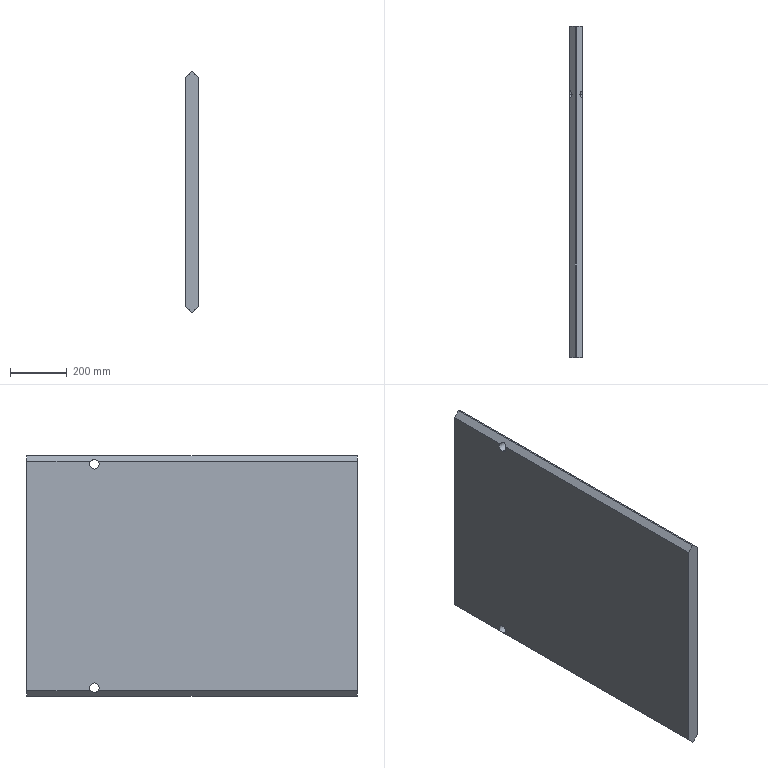Part | SolidWorks | features Chamfer 1, Extrusion 1 | 1 solid | 14 faces | box 45 x 1170 x 850 mm | volume 43736327 mm3 | plane 10 | cylinder 4 | commonest cylinder face diameters 34 x4
STEP:
#1=CARTESIAN_POINT('',(22.5,331.252,405.));
#2=VERTEX_POINT('',#1);
#3=CARTESIAN_POINT('',(22.5,345.,378.));
#4=VERTEX_POINT('',#3);
#5=CARTESIAN_POINT('',(22.5,345.,395.));
#6=DIRECTION('',(1.,0.,0.));
#7=DIRECTION('',(0.,0.,-1.));
#8=AXIS2_PLACEMENT_3D('',#5,#6,#7);
#9=CIRCLE('',#8,17.);
#10=EDGE_CURVE('',#2,#4,#9,.T.);
#11=ORIENTED_EDGE('',*,*,#10,.T.);
#12=CARTESIAN_POINT('',(-22.5,345.,378.));
#13=VERTEX_POINT('',#12);
#14=CARTESIAN_POINT('',(22.5,345.,378.));
#15=DIRECTION('',(-1.,0.,0.));
#16=VECTOR('',#15,1000.);
#17=LINE('',#14,#16);
#18=EDGE_CURVE('',#4,#13,#17,.T.);
#19=ORIENTED_EDGE('',*,*,#18,.T.);
#20=CARTESIAN_POINT('',(-22.5,331.252,405.));
#21=VERTEX_POINT('',#20);
#22=CARTESIAN_POINT('',(-22.5,345.,395.));
#23=DIRECTION('',(1.,0.,0.));
#24=DIRECTION('',(0.,0.,-1.));
#25=AXIS2_PLACEMENT_3D('',#22,#23,#24);
#26=CIRCLE('',#25,17.);
#27=EDGE_CURVE('',#21,#13,#26,.T.);
#28=ORIENTED_EDGE('',*,*,#27,.F.);
#29=CARTESIAN_POINT('',(-15.5,345.,412.));
#30=VERTEX_POINT('',#29);
#31=CARTESIAN_POINT('',(-22.5,331.252,405.));
#32=CARTESIAN_POINT('',(-18.016,334.514,409.484));
#33=CARTESIAN_POINT('',(-15.5,339.455,412.));
#34=CARTESIAN_POINT('',(-15.5,345.,412.));
#35=(BOUNDED_CURVE()B_SPLINE_CURVE(3,(#31,#32,#33,#34),.UNSPECIFIED.,.F.,.F.)B_SPLINE_CURVE_WITH_KNOTS((4,4),(2.2,3.142),.UNSPECIFIED.)CURVE()GEOMETRIC_REPRESENTATION_ITEM()RATIONAL_B_SPLINE_CURVE((1.,0.9274,0.9274,1.))REPRESENTATION_ITEM(''));
#36=EDGE_CURVE('',#21,#30,#35,.T.);
#37=ORIENTED_EDGE('',*,*,#36,.T.);
#38=CARTESIAN_POINT('',(15.5,345.,412.));
#39=VERTEX_POINT('',#38);
#40=CARTESIAN_POINT('',(22.5,345.,412.));
#41=DIRECTION('',(-1.,0.,0.));
#42=VECTOR('',#41,1000.);
#43=LINE('',#40,#42);
#44=EDGE_CURVE('',#39,#30,#43,.T.);
#45=ORIENTED_EDGE('',*,*,#44,.F.);
#46=CARTESIAN_POINT('',(15.5,345.,412.));
#47=CARTESIAN_POINT('',(15.5,339.455,412.));
#48=CARTESIAN_POINT('',(18.016,334.514,409.484));
#49=CARTESIAN_POINT('',(22.5,331.252,405.));
#50=(BOUNDED_CURVE()B_SPLINE_CURVE(3,(#46,#47,#48,#49),.UNSPECIFIED.,.F.,.T.)B_SPLINE_CURVE_WITH_KNOTS((4,4),(0.,0.9419),.UNSPECIFIED.)CURVE()GEOMETRIC_REPRESENTATION_ITEM()RATIONAL_B_SPLINE_CURVE((1.,0.9274,0.9274,1.))REPRESENTATION_ITEM(''));
#51=EDGE_CURVE('',#39,#2,#50,.T.);
#52=ORIENTED_EDGE('',*,*,#51,.T.);
#53=EDGE_LOOP('',(#11,#19,#28,#37,#45,#52));
#54=FACE_OUTER_BOUND('',#53,.T.);
#55=CARTESIAN_POINT('',(22.5,345.,395.));
#56=DIRECTION('',(-1.,0.,0.));
#57=DIRECTION('',(0.,0.,1.));
#58=AXIS2_PLACEMENT_3D('',#55,#56,#57);
#59=CYLINDRICAL_SURFACE('',#58,17.);
#60=ADVANCED_FACE('',(#54),#59,.F.);
#61=CARTESIAN_POINT('',(22.5,331.252,-405.));
#62=VERTEX_POINT('',#61);
#63=CARTESIAN_POINT('',(15.5,345.,-412.));
#64=VERTEX_POINT('',#63);
#65=CARTESIAN_POINT('',(22.5,331.252,-405.));
#66=CARTESIAN_POINT('',(18.016,334.514,-409.484));
#67=CARTESIAN_POINT('',(15.5,339.455,-412.));
#68=CARTESIAN_POINT('',(15.5,345.,-412.));
#69=(BOUNDED_CURVE()B_SPLINE_CURVE(3,(#65,#66,#67,#68),.UNSPECIFIED.,.F.,.F.)B_SPLINE_CURVE_WITH_KNOTS((4,4),(5.341,6.283),.UNSPECIFIED.)CURVE()GEOMETRIC_REPRESENTATION_ITEM()RATIONAL_B_SPLINE_CURVE((1.,0.9274,0.9274,1.))REPRESENTATION_ITEM(''));
#70=EDGE_CURVE('',#62,#64,#69,.T.);
#71=ORIENTED_EDGE('',*,*,#70,.T.);
#72=CARTESIAN_POINT('',(-15.5,345.,-412.));
#73=VERTEX_POINT('',#72);
#74=CARTESIAN_POINT('',(22.5,345.,-412.));
#75=DIRECTION('',(-1.,0.,0.));
#76=VECTOR('',#75,1000.);
#77=LINE('',#74,#76);
#78=EDGE_CURVE('',#64,#73,#77,.T.);
#79=ORIENTED_EDGE('',*,*,#78,.T.);
#80=CARTESIAN_POINT('',(-22.5,331.252,-405.));
#81=VERTEX_POINT('',#80);
#82=CARTESIAN_POINT('',(-15.5,345.,-412.));
#83=CARTESIAN_POINT('',(-15.5,339.455,-412.));
#84=CARTESIAN_POINT('',(-18.016,334.514,-409.484));
#85=CARTESIAN_POINT('',(-22.5,331.252,-405.));
#86=(BOUNDED_CURVE()B_SPLINE_CURVE(3,(#82,#83,#84,#85),.UNSPECIFIED.,.F.,.T.)B_SPLINE_CURVE_WITH_KNOTS((4,4),(3.142,4.084),.UNSPECIFIED.)CURVE()GEOMETRIC_REPRESENTATION_ITEM()RATIONAL_B_SPLINE_CURVE((1.,0.9274,0.9274,1.))REPRESENTATION_ITEM(''));
#87=EDGE_CURVE('',#73,#81,#86,.T.);
#88=ORIENTED_EDGE('',*,*,#87,.T.);
#89=CARTESIAN_POINT('',(-22.5,345.,-378.));
#90=VERTEX_POINT('',#89);
#91=CARTESIAN_POINT('',(-22.5,345.,-395.));
#92=DIRECTION('',(1.,0.,0.));
#93=DIRECTION('',(0.,0.,-1.));
#94=AXIS2_PLACEMENT_3D('',#91,#92,#93);
#95=CIRCLE('',#94,17.);
#96=EDGE_CURVE('',#90,#81,#95,.T.);
#97=ORIENTED_EDGE('',*,*,#96,.F.);
#98=CARTESIAN_POINT('',(22.5,345.,-378.));
#99=VERTEX_POINT('',#98);
#100=CARTESIAN_POINT('',(22.5,345.,-378.));
#101=DIRECTION('',(-1.,0.,0.));
#102=VECTOR('',#101,1000.);
#103=LINE('',#100,#102);
#104=EDGE_CURVE('',#99,#90,#103,.T.);
#105=ORIENTED_EDGE('',*,*,#104,.F.);
#106=CARTESIAN_POINT('',(22.5,345.,-395.));
#107=DIRECTION('',(1.,0.,0.));
#108=DIRECTION('',(0.,0.,-1.));
#109=AXIS2_PLACEMENT_3D('',#106,#107,#108);
#110=CIRCLE('',#109,17.);
#111=EDGE_CURVE('',#99,#62,#110,.T.);
#112=ORIENTED_EDGE('',*,*,#111,.T.);
#113=EDGE_LOOP('',(#71,#79,#88,#97,#105,#112));
#114=FACE_OUTER_BOUND('',#113,.T.);
#115=CARTESIAN_POINT('',(22.5,345.,-395.));
#116=DIRECTION('',(-1.,0.,0.));
#117=DIRECTION('',(0.,0.,1.));
#118=AXIS2_PLACEMENT_3D('',#115,#116,#117);
#119=CYLINDRICAL_SURFACE('',#118,17.);
#120=ADVANCED_FACE('',(#114),#119,.F.);
#121=CARTESIAN_POINT('',(22.5,-585.,405.));
#122=VERTEX_POINT('',#121);
#123=CARTESIAN_POINT('',(22.5,-585.,-405.));
#124=VERTEX_POINT('',#123);
#125=CARTESIAN_POINT('',(22.5,-585.,-425.));
#126=DIRECTION('',(0.,0.,-1.));
#127=VECTOR('',#126,1000.);
#128=LINE('',#125,#127);
#129=EDGE_CURVE('',#122,#124,#128,.T.);
#130=ORIENTED_EDGE('',*,*,#129,.T.);
#131=CARTESIAN_POINT('',(22.5,585.,-405.));
#132=DIRECTION('',(0.,1.,0.));
#133=VECTOR('',#132,1000.);
#134=LINE('',#131,#133);
#135=EDGE_CURVE('',#124,#62,#134,.T.);
#136=ORIENTED_EDGE('',*,*,#135,.T.);
#137=ORIENTED_EDGE('',*,*,#111,.F.);
#138=CARTESIAN_POINT('',(22.5,358.748,-405.));
#139=VERTEX_POINT('',#138);
#140=CARTESIAN_POINT('',(22.5,345.,-395.));
#141=DIRECTION('',(1.,0.,0.));
#142=DIRECTION('',(0.,0.,-1.));
#143=AXIS2_PLACEMENT_3D('',#140,#141,#142);
#144=CIRCLE('',#143,17.);
#145=EDGE_CURVE('',#139,#99,#144,.T.);
#146=ORIENTED_EDGE('',*,*,#145,.F.);
#147=CARTESIAN_POINT('',(22.5,585.,-405.));
#148=VERTEX_POINT('',#147);
#149=CARTESIAN_POINT('',(22.5,585.,-405.));
#150=DIRECTION('',(0.,1.,0.));
#151=VECTOR('',#150,1000.);
#152=LINE('',#149,#151);
#153=EDGE_CURVE('',#139,#148,#152,.T.);
#154=ORIENTED_EDGE('',*,*,#153,.T.);
#155=CARTESIAN_POINT('',(22.5,585.,405.));
#156=VERTEX_POINT('',#155);
#157=CARTESIAN_POINT('',(22.5,585.,-425.));
#158=DIRECTION('',(0.,0.,1.));
#159=VECTOR('',#158,1000.);
#160=LINE('',#157,#159);
#161=EDGE_CURVE('',#148,#156,#160,.T.);
#162=ORIENTED_EDGE('',*,*,#161,.T.);
#163=CARTESIAN_POINT('',(22.5,358.748,405.));
#164=VERTEX_POINT('',#163);
#165=CARTESIAN_POINT('',(22.5,-585.,405.));
#166=DIRECTION('',(0.,-1.,0.));
#167=VECTOR('',#166,1000.);
#168=LINE('',#165,#167);
#169=EDGE_CURVE('',#156,#164,#168,.T.);
#170=ORIENTED_EDGE('',*,*,#169,.T.);
#171=CARTESIAN_POINT('',(22.5,345.,395.));
#172=DIRECTION('',(1.,0.,0.));
#173=DIRECTION('',(0.,0.,-1.));
#174=AXIS2_PLACEMENT_3D('',#171,#172,#173);
#175=CIRCLE('',#174,17.);
#176=EDGE_CURVE('',#4,#164,#175,.T.);
#177=ORIENTED_EDGE('',*,*,#176,.F.);
#178=ORIENTED_EDGE('',*,*,#10,.F.);
#179=CARTESIAN_POINT('',(22.5,-585.,405.));
#180=DIRECTION('',(0.,-1.,0.));
#181=VECTOR('',#180,1000.);
#182=LINE('',#179,#181);
#183=EDGE_CURVE('',#2,#122,#182,.T.);
#184=ORIENTED_EDGE('',*,*,#183,.T.);
#185=EDGE_LOOP('',(#130,#136,#137,#146,#154,#162,#170,#177,#178,#184));
#186=FACE_OUTER_BOUND('',#185,.T.);
#187=CARTESIAN_POINT('',(22.5,0.,0.));
#188=DIRECTION('',(1.,0.,0.));
#189=DIRECTION('',(0.,0.,-1.));
#190=AXIS2_PLACEMENT_3D('',#187,#188,#189);
#191=PLANE('',#190);
#192=ADVANCED_FACE('',(#186),#191,.T.);
#193=CARTESIAN_POINT('',(-22.5,585.,-405.));
#194=VERTEX_POINT('',#193);
#195=CARTESIAN_POINT('',(-22.5,585.,405.));
#196=VERTEX_POINT('',#195);
#197=CARTESIAN_POINT('',(-22.5,585.,-425.));
#198=DIRECTION('',(0.,0.,1.));
#199=VECTOR('',#198,1000.);
#200=LINE('',#197,#199);
#201=EDGE_CURVE('',#194,#196,#200,.T.);
#202=ORIENTED_EDGE('',*,*,#201,.F.);
#203=CARTESIAN_POINT('',(-22.5,358.748,-405.));
#204=VERTEX_POINT('',#203);
#205=CARTESIAN_POINT('',(-22.5,0.,-405.));
#206=DIRECTION('',(0.,-1.,0.));
#207=VECTOR('',#206,1000.);
#208=LINE('',#205,#207);
#209=EDGE_CURVE('',#194,#204,#208,.T.);
#210=ORIENTED_EDGE('',*,*,#209,.T.);
#211=CARTESIAN_POINT('',(-22.5,345.,-395.));
#212=DIRECTION('',(1.,0.,0.));
#213=DIRECTION('',(0.,0.,-1.));
#214=AXIS2_PLACEMENT_3D('',#211,#212,#213);
#215=CIRCLE('',#214,17.);
#216=EDGE_CURVE('',#204,#90,#215,.T.);
#217=ORIENTED_EDGE('',*,*,#216,.T.);
#218=ORIENTED_EDGE('',*,*,#96,.T.);
#219=CARTESIAN_POINT('',(-22.5,-585.,-405.));
#220=VERTEX_POINT('',#219);
#221=CARTESIAN_POINT('',(-22.5,0.,-405.));
#222=DIRECTION('',(0.,-1.,0.));
#223=VECTOR('',#222,1000.);
#224=LINE('',#221,#223);
#225=EDGE_CURVE('',#81,#220,#224,.T.);
#226=ORIENTED_EDGE('',*,*,#225,.T.);
#227=CARTESIAN_POINT('',(-22.5,-585.,405.));
#228=VERTEX_POINT('',#227);
#229=CARTESIAN_POINT('',(-22.5,-585.,-425.));
#230=DIRECTION('',(0.,0.,-1.));
#231=VECTOR('',#230,1000.);
#232=LINE('',#229,#231);
#233=EDGE_CURVE('',#228,#220,#232,.T.);
#234=ORIENTED_EDGE('',*,*,#233,.F.);
#235=CARTESIAN_POINT('',(-22.5,0.,405.));
#236=DIRECTION('',(0.,1.,0.));
#237=VECTOR('',#236,1000.);
#238=LINE('',#235,#237);
#239=EDGE_CURVE('',#228,#21,#238,.T.);
#240=ORIENTED_EDGE('',*,*,#239,.T.);
#241=ORIENTED_EDGE('',*,*,#27,.T.);
#242=CARTESIAN_POINT('',(-22.5,358.748,405.));
#243=VERTEX_POINT('',#242);
#244=CARTESIAN_POINT('',(-22.5,345.,395.));
#245=DIRECTION('',(1.,0.,0.));
#246=DIRECTION('',(0.,0.,-1.));
#247=AXIS2_PLACEMENT_3D('',#244,#245,#246);
#248=CIRCLE('',#247,17.);
#249=EDGE_CURVE('',#13,#243,#248,.T.);
#250=ORIENTED_EDGE('',*,*,#249,.T.);
#251=CARTESIAN_POINT('',(-22.5,0.,405.));
#252=DIRECTION('',(0.,1.,0.));
#253=VECTOR('',#252,1000.);
#254=LINE('',#251,#253);
#255=EDGE_CURVE('',#243,#196,#254,.T.);
#256=ORIENTED_EDGE('',*,*,#255,.T.);
#257=EDGE_LOOP('',(#202,#210,#217,#218,#226,#234,#240,#241,#250,#256));
#258=FACE_OUTER_BOUND('',#257,.T.);
#259=CARTESIAN_POINT('',(-22.5,0.,0.));
#260=DIRECTION('',(1.,0.,0.));
#261=DIRECTION('',(0.,0.,-1.));
#262=AXIS2_PLACEMENT_3D('',#259,#260,#261);
#263=PLANE('',#262);
#264=ADVANCED_FACE('',(#258),#263,.F.);
#265=CARTESIAN_POINT('',(2.5,585.,425.));
#266=VERTEX_POINT('',#265);
#267=CARTESIAN_POINT('',(-2.5,585.,425.));
#268=VERTEX_POINT('',#267);
#269=CARTESIAN_POINT('',(22.5,585.,425.));
#270=DIRECTION('',(-1.,0.,0.));
#271=VECTOR('',#270,1000.);
#272=LINE('',#269,#271);
#273=EDGE_CURVE('',#266,#268,#272,.T.);
#274=ORIENTED_EDGE('',*,*,#273,.T.);
#275=CARTESIAN_POINT('',(-2.5,-585.,425.));
#276=VERTEX_POINT('',#275);
#277=CARTESIAN_POINT('',(-2.5,-585.,425.));
#278=DIRECTION('',(0.,-1.,0.));
#279=VECTOR('',#278,1000.);
#280=LINE('',#277,#279);
#281=EDGE_CURVE('',#268,#276,#280,.T.);
#282=ORIENTED_EDGE('',*,*,#281,.T.);
#283=CARTESIAN_POINT('',(2.5,-585.,425.));
#284=VERTEX_POINT('',#283);
#285=CARTESIAN_POINT('',(22.5,-585.,425.));
#286=DIRECTION('',(-1.,0.,0.));
#287=VECTOR('',#286,1000.);
#288=LINE('',#285,#287);
#289=EDGE_CURVE('',#284,#276,#288,.T.);
#290=ORIENTED_EDGE('',*,*,#289,.F.);
#291=CARTESIAN_POINT('',(2.5,585.,425.));
#292=DIRECTION('',(0.,1.,0.));
#293=VECTOR('',#292,1000.);
#294=LINE('',#291,#293);
#295=EDGE_CURVE('',#284,#266,#294,.T.);
#296=ORIENTED_EDGE('',*,*,#295,.T.);
#297=EDGE_LOOP('',(#274,#282,#290,#296));
#298=FACE_OUTER_BOUND('',#297,.T.);
#299=CARTESIAN_POINT('',(22.5,-585.,425.));
#300=DIRECTION('',(0.,0.,-1.));
#301=DIRECTION('',(-1.,0.,0.));
#302=AXIS2_PLACEMENT_3D('',#299,#300,#301);
#303=PLANE('',#302);
#304=ADVANCED_FACE('',(#298),#303,.F.);
#305=ORIENTED_EDGE('',*,*,#233,.T.);
#306=CARTESIAN_POINT('',(-2.5,-585.,-425.));
#307=VERTEX_POINT('',#306);
#308=CARTESIAN_POINT('',(-2.5,-585.,-425.));
#309=DIRECTION('',(0.7071,0.,-0.7071));
#310=VECTOR('',#309,1000.);
#311=LINE('',#308,#310);
#312=EDGE_CURVE('',#220,#307,#311,.T.);
#313=ORIENTED_EDGE('',*,*,#312,.T.);
#314=CARTESIAN_POINT('',(2.5,-585.,-425.));
#315=VERTEX_POINT('',#314);
#316=CARTESIAN_POINT('',(22.5,-585.,-425.));
#317=DIRECTION('',(-1.,0.,0.));
#318=VECTOR('',#317,1000.);
#319=LINE('',#316,#318);
#320=EDGE_CURVE('',#315,#307,#319,.T.);
#321=ORIENTED_EDGE('',*,*,#320,.F.);
#322=CARTESIAN_POINT('',(22.5,-585.,-405.));
#323=DIRECTION('',(0.7071,0.,0.7071));
#324=VECTOR('',#323,1000.);
#325=LINE('',#322,#324);
#326=EDGE_CURVE('',#315,#124,#325,.T.);
#327=ORIENTED_EDGE('',*,*,#326,.T.);
#328=ORIENTED_EDGE('',*,*,#129,.F.);
#329=CARTESIAN_POINT('',(22.5,-585.,405.));
#330=DIRECTION('',(-0.7071,0.,0.7071));
#331=VECTOR('',#330,1000.);
#332=LINE('',#329,#331);
#333=EDGE_CURVE('',#122,#284,#332,.T.);
#334=ORIENTED_EDGE('',*,*,#333,.T.);
#335=ORIENTED_EDGE('',*,*,#289,.T.);
#336=CARTESIAN_POINT('',(-2.5,-585.,425.));
#337=DIRECTION('',(-0.7071,0.,-0.7071));
#338=VECTOR('',#337,1000.);
#339=LINE('',#336,#338);
#340=EDGE_CURVE('',#276,#228,#339,.T.);
#341=ORIENTED_EDGE('',*,*,#340,.T.);
#342=EDGE_LOOP('',(#305,#313,#321,#327,#328,#334,#335,#341));
#343=FACE_OUTER_BOUND('',#342,.T.);
#344=CARTESIAN_POINT('',(22.5,-585.,-425.));
#345=DIRECTION('',(0.,1.,0.));
#346=DIRECTION('',(0.,0.,1.));
#347=AXIS2_PLACEMENT_3D('',#344,#345,#346);
#348=PLANE('',#347);
#349=ADVANCED_FACE('',(#343),#348,.F.);
#350=ORIENTED_EDGE('',*,*,#320,.T.);
#351=CARTESIAN_POINT('',(-2.5,585.,-425.));
#352=VERTEX_POINT('',#351);
#353=CARTESIAN_POINT('',(-2.5,-585.,-425.));
#354=DIRECTION('',(0.,1.,0.));
#355=VECTOR('',#354,1000.);
#356=LINE('',#353,#355);
#357=EDGE_CURVE('',#307,#352,#356,.T.);
#358=ORIENTED_EDGE('',*,*,#357,.T.);
#359=CARTESIAN_POINT('',(2.5,585.,-425.));
#360=VERTEX_POINT('',#359);
#361=CARTESIAN_POINT('',(22.5,585.,-425.));
#362=DIRECTION('',(-1.,0.,0.));
#363=VECTOR('',#362,1000.);
#364=LINE('',#361,#363);
#365=EDGE_CURVE('',#360,#352,#364,.T.);
#366=ORIENTED_EDGE('',*,*,#365,.F.);
#367=CARTESIAN_POINT('',(2.5,-585.,-425.));
#368=DIRECTION('',(0.,-1.,0.));
#369=VECTOR('',#368,1000.);
#370=LINE('',#367,#369);
#371=EDGE_CURVE('',#360,#315,#370,.T.);
#372=ORIENTED_EDGE('',*,*,#371,.T.);
#373=EDGE_LOOP('',(#350,#358,#366,#372));
#374=FACE_OUTER_BOUND('',#373,.T.);
#375=CARTESIAN_POINT('',(22.5,-585.,-425.));
#376=DIRECTION('',(0.,0.,1.));
#377=DIRECTION('',(1.,0.,0.));
#378=AXIS2_PLACEMENT_3D('',#375,#376,#377);
#379=PLANE('',#378);
#380=ADVANCED_FACE('',(#374),#379,.F.);
#381=ORIENTED_EDGE('',*,*,#365,.T.);
#382=CARTESIAN_POINT('',(-2.5,585.,-425.));
#383=DIRECTION('',(-0.7071,0.,0.7071));
#384=VECTOR('',#383,1000.);
#385=LINE('',#382,#384);
#386=EDGE_CURVE('',#352,#194,#385,.T.);
#387=ORIENTED_EDGE('',*,*,#386,.T.);
#388=ORIENTED_EDGE('',*,*,#201,.T.);
#389=CARTESIAN_POINT('',(-2.5,585.,425.));
#390=DIRECTION('',(0.7071,0.,0.7071));
#391=VECTOR('',#390,1000.);
#392=LINE('',#389,#391);
#393=EDGE_CURVE('',#196,#268,#392,.T.);
#394=ORIENTED_EDGE('',*,*,#393,.T.);
#395=ORIENTED_EDGE('',*,*,#273,.F.);
#396=CARTESIAN_POINT('',(22.5,585.,405.));
#397=DIRECTION('',(0.7071,0.,-0.7071));
#398=VECTOR('',#397,1000.);
#399=LINE('',#396,#398);
#400=EDGE_CURVE('',#266,#156,#399,.T.);
#401=ORIENTED_EDGE('',*,*,#400,.T.);
#402=ORIENTED_EDGE('',*,*,#161,.F.);
#403=CARTESIAN_POINT('',(22.5,585.,-405.));
#404=DIRECTION('',(-0.7071,0.,-0.7071));
#405=VECTOR('',#404,1000.);
#406=LINE('',#403,#405);
#407=EDGE_CURVE('',#148,#360,#406,.T.);
#408=ORIENTED_EDGE('',*,*,#407,.T.);
#409=EDGE_LOOP('',(#381,#387,#388,#394,#395,#401,#402,#408));
#410=FACE_OUTER_BOUND('',#409,.T.);
#411=CARTESIAN_POINT('',(22.5,585.,-425.));
#412=DIRECTION('',(0.,-1.,0.));
#413=DIRECTION('',(0.,0.,-1.));
#414=AXIS2_PLACEMENT_3D('',#411,#412,#413);
#415=PLANE('',#414);
#416=ADVANCED_FACE('',(#410),#415,.F.);
#417=ORIENTED_EDGE('',*,*,#78,.F.);
#418=CARTESIAN_POINT('',(15.5,345.,-412.));
#419=CARTESIAN_POINT('',(15.5,350.545,-412.));
#420=CARTESIAN_POINT('',(18.016,355.486,-409.484));
#421=CARTESIAN_POINT('',(22.5,358.748,-405.));
#422=(BOUNDED_CURVE()B_SPLINE_CURVE(3,(#418,#419,#420,#421),.UNSPECIFIED.,.F.,.T.)B_SPLINE_CURVE_WITH_KNOTS((4,4),(0.,0.9419),.UNSPECIFIED.)CURVE()GEOMETRIC_REPRESENTATION_ITEM()RATIONAL_B_SPLINE_CURVE((1.,0.9274,0.9274,1.))REPRESENTATION_ITEM(''));
#423=EDGE_CURVE('',#64,#139,#422,.T.);
#424=ORIENTED_EDGE('',*,*,#423,.T.);
#425=ORIENTED_EDGE('',*,*,#145,.T.);
#426=ORIENTED_EDGE('',*,*,#104,.T.);
#427=ORIENTED_EDGE('',*,*,#216,.F.);
#428=CARTESIAN_POINT('',(-22.5,358.748,-405.));
#429=CARTESIAN_POINT('',(-18.016,355.486,-409.484));
#430=CARTESIAN_POINT('',(-15.5,350.545,-412.));
#431=CARTESIAN_POINT('',(-15.5,345.,-412.));
#432=(BOUNDED_CURVE()B_SPLINE_CURVE(3,(#428,#429,#430,#431),.UNSPECIFIED.,.F.,.T.)B_SPLINE_CURVE_WITH_KNOTS((4,4),(2.2,3.142),.UNSPECIFIED.)CURVE()GEOMETRIC_REPRESENTATION_ITEM()RATIONAL_B_SPLINE_CURVE((1.,0.9274,0.9274,1.))REPRESENTATION_ITEM(''));
#433=EDGE_CURVE('',#204,#73,#432,.T.);
#434=ORIENTED_EDGE('',*,*,#433,.T.);
#435=EDGE_LOOP('',(#417,#424,#425,#426,#427,#434));
#436=FACE_OUTER_BOUND('',#435,.T.);
#437=CARTESIAN_POINT('',(22.5,345.,-395.));
#438=DIRECTION('',(-1.,0.,0.));
#439=DIRECTION('',(0.,0.,1.));
#440=AXIS2_PLACEMENT_3D('',#437,#438,#439);
#441=CYLINDRICAL_SURFACE('',#440,17.);
#442=ADVANCED_FACE('',(#436),#441,.F.);
#443=ORIENTED_EDGE('',*,*,#18,.F.);
#444=ORIENTED_EDGE('',*,*,#176,.T.);
#445=CARTESIAN_POINT('',(22.5,358.748,405.));
#446=CARTESIAN_POINT('',(18.016,355.486,409.484));
#447=CARTESIAN_POINT('',(15.5,350.545,412.));
#448=CARTESIAN_POINT('',(15.5,345.,412.));
#449=(BOUNDED_CURVE()B_SPLINE_CURVE(3,(#445,#446,#447,#448),.UNSPECIFIED.,.F.,.F.)B_SPLINE_CURVE_WITH_KNOTS((4,4),(5.341,6.283),.UNSPECIFIED.)CURVE()GEOMETRIC_REPRESENTATION_ITEM()RATIONAL_B_SPLINE_CURVE((1.,0.9274,0.9274,1.))REPRESENTATION_ITEM(''));
#450=EDGE_CURVE('',#164,#39,#449,.T.);
#451=ORIENTED_EDGE('',*,*,#450,.T.);
#452=ORIENTED_EDGE('',*,*,#44,.T.);
#453=CARTESIAN_POINT('',(-15.5,345.,412.));
#454=CARTESIAN_POINT('',(-15.5,350.545,412.));
#455=CARTESIAN_POINT('',(-18.016,355.486,409.484));
#456=CARTESIAN_POINT('',(-22.5,358.748,405.));
#457=(BOUNDED_CURVE()B_SPLINE_CURVE(3,(#453,#454,#455,#456),.UNSPECIFIED.,.F.,.F.)B_SPLINE_CURVE_WITH_KNOTS((4,4),(3.142,4.084),.UNSPECIFIED.)CURVE()GEOMETRIC_REPRESENTATION_ITEM()RATIONAL_B_SPLINE_CURVE((1.,0.9274,0.9274,1.))REPRESENTATION_ITEM(''));
#458=EDGE_CURVE('',#30,#243,#457,.T.);
#459=ORIENTED_EDGE('',*,*,#458,.T.);
#460=ORIENTED_EDGE('',*,*,#249,.F.);
#461=EDGE_LOOP('',(#443,#444,#451,#452,#459,#460));
#462=FACE_OUTER_BOUND('',#461,.T.);
#463=CARTESIAN_POINT('',(22.5,345.,395.));
#464=DIRECTION('',(-1.,0.,0.));
#465=DIRECTION('',(0.,0.,1.));
#466=AXIS2_PLACEMENT_3D('',#463,#464,#465);
#467=CYLINDRICAL_SURFACE('',#466,17.);
#468=ADVANCED_FACE('',(#462),#467,.F.);
#469=ORIENTED_EDGE('',*,*,#433,.F.);
#470=ORIENTED_EDGE('',*,*,#209,.F.);
#471=ORIENTED_EDGE('',*,*,#386,.F.);
#472=ORIENTED_EDGE('',*,*,#357,.F.);
#473=ORIENTED_EDGE('',*,*,#312,.F.);
#474=ORIENTED_EDGE('',*,*,#225,.F.);
#475=ORIENTED_EDGE('',*,*,#87,.F.);
#476=EDGE_LOOP('',(#469,#470,#471,#472,#473,#474,#475));
#477=FACE_OUTER_BOUND('',#476,.T.);
#478=CARTESIAN_POINT('',(-2.5,-585.,-425.));
#479=DIRECTION('',(0.7071,0.,0.7071));
#480=DIRECTION('',(0.,1.,0.));
#481=AXIS2_PLACEMENT_3D('',#478,#479,#480);
#482=PLANE('',#481);
#483=ADVANCED_FACE('',(#477),#482,.F.);
#484=ORIENTED_EDGE('',*,*,#326,.F.);
#485=ORIENTED_EDGE('',*,*,#371,.F.);
#486=ORIENTED_EDGE('',*,*,#407,.F.);
#487=ORIENTED_EDGE('',*,*,#153,.F.);
#488=ORIENTED_EDGE('',*,*,#423,.F.);
#489=ORIENTED_EDGE('',*,*,#70,.F.);
#490=ORIENTED_EDGE('',*,*,#135,.F.);
#491=EDGE_LOOP('',(#484,#485,#486,#487,#488,#489,#490));
#492=FACE_OUTER_BOUND('',#491,.T.);
#493=CARTESIAN_POINT('',(22.5,0.,-405.));
#494=DIRECTION('',(0.7071,0.,-0.7071));
#495=DIRECTION('',(0.,-1.,0.));
#496=AXIS2_PLACEMENT_3D('',#493,#494,#495);
#497=PLANE('',#496);
#498=ADVANCED_FACE('',(#492),#497,.T.);
#499=ORIENTED_EDGE('',*,*,#36,.F.);
#500=ORIENTED_EDGE('',*,*,#239,.F.);
#501=ORIENTED_EDGE('',*,*,#340,.F.);
#502=ORIENTED_EDGE('',*,*,#281,.F.);
#503=ORIENTED_EDGE('',*,*,#393,.F.);
#504=ORIENTED_EDGE('',*,*,#255,.F.);
#505=ORIENTED_EDGE('',*,*,#458,.F.);
#506=EDGE_LOOP('',(#499,#500,#501,#502,#503,#504,#505));
#507=FACE_OUTER_BOUND('',#506,.T.);
#508=CARTESIAN_POINT('',(-2.5,-585.,425.));
#509=DIRECTION('',(0.7071,0.,-0.7071));
#510=DIRECTION('',(0.,-1.,0.));
#511=AXIS2_PLACEMENT_3D('',#508,#509,#510);
#512=PLANE('',#511);
#513=ADVANCED_FACE('',(#507),#512,.F.);
#514=ORIENTED_EDGE('',*,*,#400,.F.);
#515=ORIENTED_EDGE('',*,*,#295,.F.);
#516=ORIENTED_EDGE('',*,*,#333,.F.);
#517=ORIENTED_EDGE('',*,*,#183,.F.);
#518=ORIENTED_EDGE('',*,*,#51,.F.);
#519=ORIENTED_EDGE('',*,*,#450,.F.);
#520=ORIENTED_EDGE('',*,*,#169,.F.);
#521=EDGE_LOOP('',(#514,#515,#516,#517,#518,#519,#520));
#522=FACE_OUTER_BOUND('',#521,.T.);
#523=CARTESIAN_POINT('',(22.5,0.,405.));
#524=DIRECTION('',(0.7071,0.,0.7071));
#525=DIRECTION('',(0.,1.,0.));
#526=AXIS2_PLACEMENT_3D('',#523,#524,#525);
#527=PLANE('',#526);
#528=ADVANCED_FACE('',(#522),#527,.T.);
#529=CLOSED_SHELL('',(#60,#120,#192,#264,#304,#349,#380,#416,#442,#468,#483,#498,#513,#528));
#530=MANIFOLD_SOLID_BREP('',#529);
#531=CARTESIAN_POINT('',(0.,0.,0.));
#532=DIRECTION('',(0.,0.,1.));
#533=DIRECTION('',(1.,0.,0.));
#534=AXIS2_PLACEMENT_3D('',#531,#532,#533);
#535=(LENGTH_UNIT()NAMED_UNIT(*)SI_UNIT(.MILLI.,.METRE.));
#536=UNCERTAINTY_MEASURE_WITH_UNIT(LENGTH_MEASURE(0.00001),#535,'','');
#537=(NAMED_UNIT(*)PLANE_ANGLE_UNIT()SI_UNIT($,.RADIAN.));
#538=(NAMED_UNIT(*)SI_UNIT($,.STERADIAN.)SOLID_ANGLE_UNIT());
#539=(GEOMETRIC_REPRESENTATION_CONTEXT(3)GLOBAL_UNCERTAINTY_ASSIGNED_CONTEXT((#536))GLOBAL_UNIT_ASSIGNED_CONTEXT((#535,#537,#538))REPRESENTATION_CONTEXT('',''));
#540=ADVANCED_BREP_SHAPE_REPRESENTATION('',(#530,#534),#539);